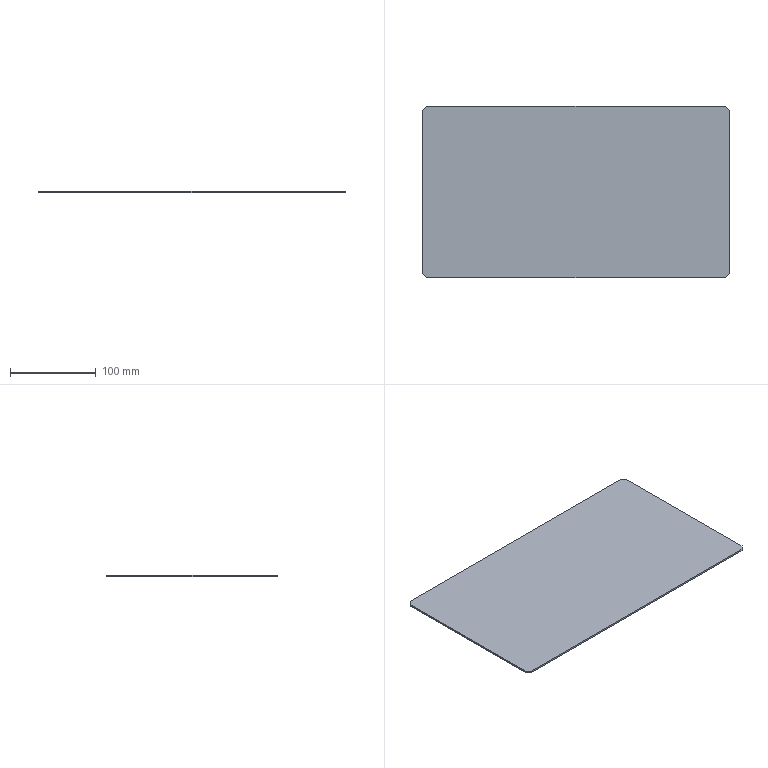Part | STEP file | PN_0042 | 1 solid | 10 faces | box 358 x 200 x 2 mm | volume 143100 mm3 | plane 10
STEP:
#1=CARTESIAN_POINT('',(0.,0.,0.));
#2=DIRECTION('',(0.,0.,1.));
#3=DIRECTION('',(1.,0.,0.));
#4=AXIS2_PLACEMENT_3D('',#1,#2,#3);
#5=CARTESIAN_POINT('',(179.,-95.,2.));
#6=VERTEX_POINT('',#5);
#7=CARTESIAN_POINT('',(179.,95.,2.));
#8=VERTEX_POINT('',#7);
#9=CARTESIAN_POINT('',(179.,100.,2.));
#10=DIRECTION('',(0.,1.,0.));
#11=VECTOR('',#10,1.);
#12=LINE('',#9,#11);
#13=CARTESIAN_POINT('',(179.,100.,2.));
#14=DIRECTION('',(-1.,0.,0.));
#15=DIRECTION('',(0.,-1.,0.));
#16=AXIS2_PLACEMENT_3D('',#13,#14,#15);
#17=PLANE('',#16);
#18=CARTESIAN_POINT('',(0.,0.));
#19=DIRECTION('',(-1.,0.));
#20=VECTOR('',#19,1.);
#21=LINE('',#18,#20);
#22=(GEOMETRIC_REPRESENTATION_CONTEXT(2)PARAMETRIC_REPRESENTATION_CONTEXT()REPRESENTATION_CONTEXT('',''));
#23=DEFINITIONAL_REPRESENTATION('',(#21),#22);
#24=PCURVE('',#17,#23);
#25=CARTESIAN_POINT('',(179.,-100.,2.));
#26=DIRECTION('',(0.,0.,1.));
#27=DIRECTION('',(1.,0.,0.));
#28=AXIS2_PLACEMENT_3D('',#25,#26,#27);
#29=PLANE('',#28);
#30=CARTESIAN_POINT('',(0.,200.));
#31=DIRECTION('',(0.,1.));
#32=VECTOR('',#31,1.);
#33=LINE('',#30,#32);
#34=(GEOMETRIC_REPRESENTATION_CONTEXT(2)PARAMETRIC_REPRESENTATION_CONTEXT()REPRESENTATION_CONTEXT('',''));
#35=DEFINITIONAL_REPRESENTATION('',(#33),#34);
#36=PCURVE('',#29,#35);
#37=SURFACE_CURVE('',#12,(#24,#36),.PCURVE_S1.);
#38=EDGE_CURVE('',#6,#8,#37,.T.);
#39=ORIENTED_EDGE('',*,*,#38,.F.);
#40=CARTESIAN_POINT('',(179.,-95.,0.));
#41=VERTEX_POINT('',#40);
#42=CARTESIAN_POINT('',(179.,-95.,2.));
#43=DIRECTION('',(0.,0.,-1.));
#44=VECTOR('',#43,1.);
#45=LINE('',#42,#44);
#46=CARTESIAN_POINT('',(195.,0.));
#47=DIRECTION('',(0.,-1.));
#48=VECTOR('',#47,1.);
#49=LINE('',#46,#48);
#50=(GEOMETRIC_REPRESENTATION_CONTEXT(2)PARAMETRIC_REPRESENTATION_CONTEXT()REPRESENTATION_CONTEXT('',''));
#51=DEFINITIONAL_REPRESENTATION('',(#49),#50);
#52=PCURVE('',#17,#51);
#53=CARTESIAN_POINT('',(179.,-95.,2.));
#54=DIRECTION('',(-0.7071,0.7071,0.));
#55=DIRECTION('',(-0.7071,-0.7071,0.));
#56=AXIS2_PLACEMENT_3D('',#53,#54,#55);
#57=PLANE('',#56);
#58=CARTESIAN_POINT('',(0.,0.));
#59=DIRECTION('',(0.,-1.));
#60=VECTOR('',#59,1.);
#61=LINE('',#58,#60);
#62=(GEOMETRIC_REPRESENTATION_CONTEXT(2)PARAMETRIC_REPRESENTATION_CONTEXT()REPRESENTATION_CONTEXT('',''));
#63=DEFINITIONAL_REPRESENTATION('',(#61),#62);
#64=PCURVE('',#57,#63);
#65=SURFACE_CURVE('',#45,(#52,#64),.PCURVE_S1.);
#66=EDGE_CURVE('',#6,#41,#65,.T.);
#67=ORIENTED_EDGE('',*,*,#66,.T.);
#68=CARTESIAN_POINT('',(179.,95.,0.));
#69=VERTEX_POINT('',#68);
#70=CARTESIAN_POINT('',(179.,100.,0.));
#71=DIRECTION('',(0.,1.,0.));
#72=VECTOR('',#71,1.);
#73=LINE('',#70,#72);
#74=CARTESIAN_POINT('',(0.,-2.));
#75=DIRECTION('',(-1.,0.));
#76=VECTOR('',#75,1.);
#77=LINE('',#74,#76);
#78=(GEOMETRIC_REPRESENTATION_CONTEXT(2)PARAMETRIC_REPRESENTATION_CONTEXT()REPRESENTATION_CONTEXT('',''));
#79=DEFINITIONAL_REPRESENTATION('',(#77),#78);
#80=PCURVE('',#17,#79);
#81=CARTESIAN_POINT('',(179.,-100.,0.));
#82=DIRECTION('',(0.,0.,1.));
#83=DIRECTION('',(1.,0.,0.));
#84=AXIS2_PLACEMENT_3D('',#81,#82,#83);
#85=PLANE('',#84);
#86=CARTESIAN_POINT('',(0.,200.));
#87=DIRECTION('',(0.,1.));
#88=VECTOR('',#87,1.);
#89=LINE('',#86,#88);
#90=(GEOMETRIC_REPRESENTATION_CONTEXT(2)PARAMETRIC_REPRESENTATION_CONTEXT()REPRESENTATION_CONTEXT('',''));
#91=DEFINITIONAL_REPRESENTATION('',(#89),#90);
#92=PCURVE('',#85,#91);
#93=SURFACE_CURVE('',#73,(#80,#92),.PCURVE_S1.);
#94=EDGE_CURVE('',#41,#69,#93,.T.);
#95=ORIENTED_EDGE('',*,*,#94,.T.);
#96=CARTESIAN_POINT('',(179.,95.,2.));
#97=DIRECTION('',(0.,0.,1.));
#98=VECTOR('',#97,1.);
#99=LINE('',#96,#98);
#100=CARTESIAN_POINT('',(5.,0.));
#101=DIRECTION('',(0.,1.));
#102=VECTOR('',#101,1.);
#103=LINE('',#100,#102);
#104=(GEOMETRIC_REPRESENTATION_CONTEXT(2)PARAMETRIC_REPRESENTATION_CONTEXT()REPRESENTATION_CONTEXT('',''));
#105=DEFINITIONAL_REPRESENTATION('',(#103),#104);
#106=PCURVE('',#17,#105);
#107=CARTESIAN_POINT('',(174.,100.,2.));
#108=DIRECTION('',(-0.7071,-0.7071,0.));
#109=DIRECTION('',(0.7071,-0.7071,0.));
#110=AXIS2_PLACEMENT_3D('',#107,#108,#109);
#111=PLANE('',#110);
#112=CARTESIAN_POINT('',(7.071,0.));
#113=DIRECTION('',(0.,1.));
#114=VECTOR('',#113,1.);
#115=LINE('',#112,#114);
#116=(GEOMETRIC_REPRESENTATION_CONTEXT(2)PARAMETRIC_REPRESENTATION_CONTEXT()REPRESENTATION_CONTEXT('',''));
#117=DEFINITIONAL_REPRESENTATION('',(#115),#116);
#118=PCURVE('',#111,#117);
#119=SURFACE_CURVE('',#99,(#106,#118),.PCURVE_S1.);
#120=EDGE_CURVE('',#69,#8,#119,.T.);
#121=ORIENTED_EDGE('',*,*,#120,.T.);
#122=EDGE_LOOP('',(#39,#67,#95,#121));
#123=FACE_BOUND('',#122,.T.);
#124=ADVANCED_FACE('',(#123),#17,.F.);
#125=CARTESIAN_POINT('',(174.,100.,0.));
#126=VERTEX_POINT('',#125);
#127=CARTESIAN_POINT('',(-174.,100.,0.));
#128=VERTEX_POINT('',#127);
#129=CARTESIAN_POINT('',(-179.,100.,0.));
#130=DIRECTION('',(-1.,0.,0.));
#131=VECTOR('',#130,1.);
#132=LINE('',#129,#131);
#133=CARTESIAN_POINT('',(-179.,100.,2.));
#134=DIRECTION('',(0.,-1.,0.));
#135=DIRECTION('',(0.,0.,-1.));
#136=AXIS2_PLACEMENT_3D('',#133,#134,#135);
#137=PLANE('',#136);
#138=CARTESIAN_POINT('',(2.,0.));
#139=DIRECTION('',(0.,-1.));
#140=VECTOR('',#139,1.);
#141=LINE('',#138,#140);
#142=(GEOMETRIC_REPRESENTATION_CONTEXT(2)PARAMETRIC_REPRESENTATION_CONTEXT()REPRESENTATION_CONTEXT('',''));
#143=DEFINITIONAL_REPRESENTATION('',(#141),#142);
#144=PCURVE('',#137,#143);
#145=CARTESIAN_POINT('',(-358.,200.));
#146=DIRECTION('',(-1.,0.));
#147=VECTOR('',#146,1.);
#148=LINE('',#145,#147);
#149=(GEOMETRIC_REPRESENTATION_CONTEXT(2)PARAMETRIC_REPRESENTATION_CONTEXT()REPRESENTATION_CONTEXT('',''));
#150=DEFINITIONAL_REPRESENTATION('',(#148),#149);
#151=PCURVE('',#85,#150);
#152=SURFACE_CURVE('',#132,(#144,#151),.PCURVE_S1.);
#153=EDGE_CURVE('',#126,#128,#152,.T.);
#154=ORIENTED_EDGE('',*,*,#153,.T.);
#155=CARTESIAN_POINT('',(-174.,100.,2.));
#156=VERTEX_POINT('',#155);
#157=CARTESIAN_POINT('',(-174.,100.,2.));
#158=DIRECTION('',(0.,0.,1.));
#159=VECTOR('',#158,1.);
#160=LINE('',#157,#159);
#161=CARTESIAN_POINT('',(0.,5.));
#162=DIRECTION('',(-1.,0.));
#163=VECTOR('',#162,1.);
#164=LINE('',#161,#163);
#165=(GEOMETRIC_REPRESENTATION_CONTEXT(2)PARAMETRIC_REPRESENTATION_CONTEXT()REPRESENTATION_CONTEXT('',''));
#166=DEFINITIONAL_REPRESENTATION('',(#164),#165);
#167=PCURVE('',#137,#166);
#168=CARTESIAN_POINT('',(-179.,95.,2.));
#169=DIRECTION('',(0.7071,-0.7071,0.));
#170=DIRECTION('',(0.7071,0.7071,0.));
#171=AXIS2_PLACEMENT_3D('',#168,#169,#170);
#172=PLANE('',#171);
#173=CARTESIAN_POINT('',(7.071,0.));
#174=DIRECTION('',(0.,1.));
#175=VECTOR('',#174,1.);
#176=LINE('',#173,#175);
#177=(GEOMETRIC_REPRESENTATION_CONTEXT(2)PARAMETRIC_REPRESENTATION_CONTEXT()REPRESENTATION_CONTEXT('',''));
#178=DEFINITIONAL_REPRESENTATION('',(#176),#177);
#179=PCURVE('',#172,#178);
#180=SURFACE_CURVE('',#160,(#167,#179),.PCURVE_S1.);
#181=EDGE_CURVE('',#128,#156,#180,.T.);
#182=ORIENTED_EDGE('',*,*,#181,.T.);
#183=CARTESIAN_POINT('',(174.,100.,2.));
#184=VERTEX_POINT('',#183);
#185=CARTESIAN_POINT('',(-179.,100.,2.));
#186=DIRECTION('',(-1.,0.,0.));
#187=VECTOR('',#186,1.);
#188=LINE('',#185,#187);
#189=CARTESIAN_POINT('',(0.,0.));
#190=DIRECTION('',(0.,-1.));
#191=VECTOR('',#190,1.);
#192=LINE('',#189,#191);
#193=(GEOMETRIC_REPRESENTATION_CONTEXT(2)PARAMETRIC_REPRESENTATION_CONTEXT()REPRESENTATION_CONTEXT('',''));
#194=DEFINITIONAL_REPRESENTATION('',(#192),#193);
#195=PCURVE('',#137,#194);
#196=CARTESIAN_POINT('',(-358.,200.));
#197=DIRECTION('',(-1.,0.));
#198=VECTOR('',#197,1.);
#199=LINE('',#196,#198);
#200=(GEOMETRIC_REPRESENTATION_CONTEXT(2)PARAMETRIC_REPRESENTATION_CONTEXT()REPRESENTATION_CONTEXT('',''));
#201=DEFINITIONAL_REPRESENTATION('',(#199),#200);
#202=PCURVE('',#29,#201);
#203=SURFACE_CURVE('',#188,(#195,#202),.PCURVE_S1.);
#204=EDGE_CURVE('',#184,#156,#203,.T.);
#205=ORIENTED_EDGE('',*,*,#204,.F.);
#206=CARTESIAN_POINT('',(174.,100.,2.));
#207=DIRECTION('',(0.,0.,-1.));
#208=VECTOR('',#207,1.);
#209=LINE('',#206,#208);
#210=CARTESIAN_POINT('',(0.,353.));
#211=DIRECTION('',(1.,0.));
#212=VECTOR('',#211,1.);
#213=LINE('',#210,#212);
#214=(GEOMETRIC_REPRESENTATION_CONTEXT(2)PARAMETRIC_REPRESENTATION_CONTEXT()REPRESENTATION_CONTEXT('',''));
#215=DEFINITIONAL_REPRESENTATION('',(#213),#214);
#216=PCURVE('',#137,#215);
#217=CARTESIAN_POINT('',(0.,0.));
#218=DIRECTION('',(0.,-1.));
#219=VECTOR('',#218,1.);
#220=LINE('',#217,#219);
#221=(GEOMETRIC_REPRESENTATION_CONTEXT(2)PARAMETRIC_REPRESENTATION_CONTEXT()REPRESENTATION_CONTEXT('',''));
#222=DEFINITIONAL_REPRESENTATION('',(#220),#221);
#223=PCURVE('',#111,#222);
#224=SURFACE_CURVE('',#209,(#216,#223),.PCURVE_S1.);
#225=EDGE_CURVE('',#184,#126,#224,.T.);
#226=ORIENTED_EDGE('',*,*,#225,.T.);
#227=EDGE_LOOP('',(#154,#182,#205,#226));
#228=FACE_BOUND('',#227,.T.);
#229=ADVANCED_FACE('',(#228),#137,.F.);
#230=CARTESIAN_POINT('',(-179.,95.,0.));
#231=VERTEX_POINT('',#230);
#232=CARTESIAN_POINT('',(-179.,-95.,0.));
#233=VERTEX_POINT('',#232);
#234=CARTESIAN_POINT('',(-179.,100.,0.));
#235=DIRECTION('',(0.,-1.,0.));
#236=VECTOR('',#235,1.);
#237=LINE('',#234,#236);
#238=CARTESIAN_POINT('',(-179.,100.,2.));
#239=DIRECTION('',(1.,0.,0.));
#240=DIRECTION('',(0.,1.,0.));
#241=AXIS2_PLACEMENT_3D('',#238,#239,#240);
#242=PLANE('',#241);
#243=CARTESIAN_POINT('',(0.,-2.));
#244=DIRECTION('',(-1.,0.));
#245=VECTOR('',#244,1.);
#246=LINE('',#243,#245);
#247=(GEOMETRIC_REPRESENTATION_CONTEXT(2)PARAMETRIC_REPRESENTATION_CONTEXT()REPRESENTATION_CONTEXT('',''));
#248=DEFINITIONAL_REPRESENTATION('',(#246),#247);
#249=PCURVE('',#242,#248);
#250=CARTESIAN_POINT('',(-358.,200.));
#251=DIRECTION('',(0.,-1.));
#252=VECTOR('',#251,1.);
#253=LINE('',#250,#252);
#254=(GEOMETRIC_REPRESENTATION_CONTEXT(2)PARAMETRIC_REPRESENTATION_CONTEXT()REPRESENTATION_CONTEXT('',''));
#255=DEFINITIONAL_REPRESENTATION('',(#253),#254);
#256=PCURVE('',#85,#255);
#257=SURFACE_CURVE('',#237,(#249,#256),.PCURVE_S1.);
#258=EDGE_CURVE('',#231,#233,#257,.T.);
#259=ORIENTED_EDGE('',*,*,#258,.T.);
#260=CARTESIAN_POINT('',(-179.,-95.,2.));
#261=VERTEX_POINT('',#260);
#262=CARTESIAN_POINT('',(-179.,-95.,2.));
#263=DIRECTION('',(0.,0.,1.));
#264=VECTOR('',#263,1.);
#265=LINE('',#262,#264);
#266=CARTESIAN_POINT('',(-195.,0.));
#267=DIRECTION('',(0.,1.));
#268=VECTOR('',#267,1.);
#269=LINE('',#266,#268);
#270=(GEOMETRIC_REPRESENTATION_CONTEXT(2)PARAMETRIC_REPRESENTATION_CONTEXT()REPRESENTATION_CONTEXT('',''));
#271=DEFINITIONAL_REPRESENTATION('',(#269),#270);
#272=PCURVE('',#242,#271);
#273=CARTESIAN_POINT('',(-174.,-100.,2.));
#274=DIRECTION('',(0.7071,0.7071,0.));
#275=DIRECTION('',(-0.7071,0.7071,0.));
#276=AXIS2_PLACEMENT_3D('',#273,#274,#275);
#277=PLANE('',#276);
#278=CARTESIAN_POINT('',(7.071,0.));
#279=DIRECTION('',(0.,1.));
#280=VECTOR('',#279,1.);
#281=LINE('',#278,#280);
#282=(GEOMETRIC_REPRESENTATION_CONTEXT(2)PARAMETRIC_REPRESENTATION_CONTEXT()REPRESENTATION_CONTEXT('',''));
#283=DEFINITIONAL_REPRESENTATION('',(#281),#282);
#284=PCURVE('',#277,#283);
#285=SURFACE_CURVE('',#265,(#272,#284),.PCURVE_S1.);
#286=EDGE_CURVE('',#233,#261,#285,.T.);
#287=ORIENTED_EDGE('',*,*,#286,.T.);
#288=CARTESIAN_POINT('',(-179.,95.,2.));
#289=VERTEX_POINT('',#288);
#290=CARTESIAN_POINT('',(-179.,100.,2.));
#291=DIRECTION('',(0.,-1.,0.));
#292=VECTOR('',#291,1.);
#293=LINE('',#290,#292);
#294=CARTESIAN_POINT('',(0.,0.));
#295=DIRECTION('',(-1.,0.));
#296=VECTOR('',#295,1.);
#297=LINE('',#294,#296);
#298=(GEOMETRIC_REPRESENTATION_CONTEXT(2)PARAMETRIC_REPRESENTATION_CONTEXT()REPRESENTATION_CONTEXT('',''));
#299=DEFINITIONAL_REPRESENTATION('',(#297),#298);
#300=PCURVE('',#242,#299);
#301=CARTESIAN_POINT('',(-358.,200.));
#302=DIRECTION('',(0.,-1.));
#303=VECTOR('',#302,1.);
#304=LINE('',#301,#303);
#305=(GEOMETRIC_REPRESENTATION_CONTEXT(2)PARAMETRIC_REPRESENTATION_CONTEXT()REPRESENTATION_CONTEXT('',''));
#306=DEFINITIONAL_REPRESENTATION('',(#304),#305);
#307=PCURVE('',#29,#306);
#308=SURFACE_CURVE('',#293,(#300,#307),.PCURVE_S1.);
#309=EDGE_CURVE('',#289,#261,#308,.T.);
#310=ORIENTED_EDGE('',*,*,#309,.F.);
#311=CARTESIAN_POINT('',(-179.,95.,2.));
#312=DIRECTION('',(0.,0.,-1.));
#313=VECTOR('',#312,1.);
#314=LINE('',#311,#313);
#315=CARTESIAN_POINT('',(-5.,0.));
#316=DIRECTION('',(0.,-1.));
#317=VECTOR('',#316,1.);
#318=LINE('',#315,#317);
#319=(GEOMETRIC_REPRESENTATION_CONTEXT(2)PARAMETRIC_REPRESENTATION_CONTEXT()REPRESENTATION_CONTEXT('',''));
#320=DEFINITIONAL_REPRESENTATION('',(#318),#319);
#321=PCURVE('',#242,#320);
#322=CARTESIAN_POINT('',(0.,0.));
#323=DIRECTION('',(0.,-1.));
#324=VECTOR('',#323,1.);
#325=LINE('',#322,#324);
#326=(GEOMETRIC_REPRESENTATION_CONTEXT(2)PARAMETRIC_REPRESENTATION_CONTEXT()REPRESENTATION_CONTEXT('',''));
#327=DEFINITIONAL_REPRESENTATION('',(#325),#326);
#328=PCURVE('',#172,#327);
#329=SURFACE_CURVE('',#314,(#321,#328),.PCURVE_S1.);
#330=EDGE_CURVE('',#289,#231,#329,.T.);
#331=ORIENTED_EDGE('',*,*,#330,.T.);
#332=EDGE_LOOP('',(#259,#287,#310,#331));
#333=FACE_BOUND('',#332,.T.);
#334=ADVANCED_FACE('',(#333),#242,.F.);
#335=CARTESIAN_POINT('',(-174.,-100.,2.));
#336=VERTEX_POINT('',#335);
#337=CARTESIAN_POINT('',(174.,-100.,2.));
#338=VERTEX_POINT('',#337);
#339=CARTESIAN_POINT('',(-179.,-100.,2.));
#340=DIRECTION('',(1.,0.,0.));
#341=VECTOR('',#340,1.);
#342=LINE('',#339,#341);
#343=CARTESIAN_POINT('',(-179.,-100.,2.));
#344=DIRECTION('',(0.,1.,0.));
#345=DIRECTION('',(0.,0.,1.));
#346=AXIS2_PLACEMENT_3D('',#343,#344,#345);
#347=PLANE('',#346);
#348=CARTESIAN_POINT('',(0.,0.));
#349=DIRECTION('',(0.,1.));
#350=VECTOR('',#349,1.);
#351=LINE('',#348,#350);
#352=(GEOMETRIC_REPRESENTATION_CONTEXT(2)PARAMETRIC_REPRESENTATION_CONTEXT()REPRESENTATION_CONTEXT('',''));
#353=DEFINITIONAL_REPRESENTATION('',(#351),#352);
#354=PCURVE('',#347,#353);
#355=CARTESIAN_POINT('',(-358.,0.));
#356=DIRECTION('',(1.,0.));
#357=VECTOR('',#356,1.);
#358=LINE('',#355,#357);
#359=(GEOMETRIC_REPRESENTATION_CONTEXT(2)PARAMETRIC_REPRESENTATION_CONTEXT()REPRESENTATION_CONTEXT('',''));
#360=DEFINITIONAL_REPRESENTATION('',(#358),#359);
#361=PCURVE('',#29,#360);
#362=SURFACE_CURVE('',#342,(#354,#361),.PCURVE_S1.);
#363=EDGE_CURVE('',#336,#338,#362,.T.);
#364=ORIENTED_EDGE('',*,*,#363,.F.);
#365=CARTESIAN_POINT('',(-174.,-100.,0.));
#366=VERTEX_POINT('',#365);
#367=CARTESIAN_POINT('',(-174.,-100.,2.));
#368=DIRECTION('',(0.,0.,-1.));
#369=VECTOR('',#368,1.);
#370=LINE('',#367,#369);
#371=CARTESIAN_POINT('',(0.,5.));
#372=DIRECTION('',(-1.,0.));
#373=VECTOR('',#372,1.);
#374=LINE('',#371,#373);
#375=(GEOMETRIC_REPRESENTATION_CONTEXT(2)PARAMETRIC_REPRESENTATION_CONTEXT()REPRESENTATION_CONTEXT('',''));
#376=DEFINITIONAL_REPRESENTATION('',(#374),#375);
#377=PCURVE('',#347,#376);
#378=CARTESIAN_POINT('',(0.,0.));
#379=DIRECTION('',(0.,-1.));
#380=VECTOR('',#379,1.);
#381=LINE('',#378,#380);
#382=(GEOMETRIC_REPRESENTATION_CONTEXT(2)PARAMETRIC_REPRESENTATION_CONTEXT()REPRESENTATION_CONTEXT('',''));
#383=DEFINITIONAL_REPRESENTATION('',(#381),#382);
#384=PCURVE('',#277,#383);
#385=SURFACE_CURVE('',#370,(#377,#384),.PCURVE_S1.);
#386=EDGE_CURVE('',#336,#366,#385,.T.);
#387=ORIENTED_EDGE('',*,*,#386,.T.);
#388=CARTESIAN_POINT('',(174.,-100.,0.));
#389=VERTEX_POINT('',#388);
#390=CARTESIAN_POINT('',(-179.,-100.,0.));
#391=DIRECTION('',(1.,0.,0.));
#392=VECTOR('',#391,1.);
#393=LINE('',#390,#392);
#394=CARTESIAN_POINT('',(-2.,0.));
#395=DIRECTION('',(0.,1.));
#396=VECTOR('',#395,1.);
#397=LINE('',#394,#396);
#398=(GEOMETRIC_REPRESENTATION_CONTEXT(2)PARAMETRIC_REPRESENTATION_CONTEXT()REPRESENTATION_CONTEXT('',''));
#399=DEFINITIONAL_REPRESENTATION('',(#397),#398);
#400=PCURVE('',#347,#399);
#401=CARTESIAN_POINT('',(-358.,0.));
#402=DIRECTION('',(1.,0.));
#403=VECTOR('',#402,1.);
#404=LINE('',#401,#403);
#405=(GEOMETRIC_REPRESENTATION_CONTEXT(2)PARAMETRIC_REPRESENTATION_CONTEXT()REPRESENTATION_CONTEXT('',''));
#406=DEFINITIONAL_REPRESENTATION('',(#404),#405);
#407=PCURVE('',#85,#406);
#408=SURFACE_CURVE('',#393,(#400,#407),.PCURVE_S1.);
#409=EDGE_CURVE('',#366,#389,#408,.T.);
#410=ORIENTED_EDGE('',*,*,#409,.T.);
#411=CARTESIAN_POINT('',(174.,-100.,2.));
#412=DIRECTION('',(0.,0.,1.));
#413=VECTOR('',#412,1.);
#414=LINE('',#411,#413);
#415=CARTESIAN_POINT('',(0.,353.));
#416=DIRECTION('',(1.,0.));
#417=VECTOR('',#416,1.);
#418=LINE('',#415,#417);
#419=(GEOMETRIC_REPRESENTATION_CONTEXT(2)PARAMETRIC_REPRESENTATION_CONTEXT()REPRESENTATION_CONTEXT('',''));
#420=DEFINITIONAL_REPRESENTATION('',(#418),#419);
#421=PCURVE('',#347,#420);
#422=CARTESIAN_POINT('',(7.071,0.));
#423=DIRECTION('',(0.,1.));
#424=VECTOR('',#423,1.);
#425=LINE('',#422,#424);
#426=(GEOMETRIC_REPRESENTATION_CONTEXT(2)PARAMETRIC_REPRESENTATION_CONTEXT()REPRESENTATION_CONTEXT('',''));
#427=DEFINITIONAL_REPRESENTATION('',(#425),#426);
#428=PCURVE('',#57,#427);
#429=SURFACE_CURVE('',#414,(#421,#428),.PCURVE_S1.);
#430=EDGE_CURVE('',#389,#338,#429,.T.);
#431=ORIENTED_EDGE('',*,*,#430,.T.);
#432=EDGE_LOOP('',(#364,#387,#410,#431));
#433=FACE_BOUND('',#432,.T.);
#434=ADVANCED_FACE('',(#433),#347,.F.);
#435=ORIENTED_EDGE('',*,*,#309,.T.);
#436=CARTESIAN_POINT('',(2.5,-276.5,2.));
#437=DIRECTION('',(0.7071,-0.7071,0.));
#438=VECTOR('',#437,1.);
#439=LINE('',#436,#438);
#440=CARTESIAN_POINT('',(-176.5,-176.5));
#441=DIRECTION('',(0.7071,-0.7071));
#442=VECTOR('',#441,1.);
#443=LINE('',#440,#442);
#444=(GEOMETRIC_REPRESENTATION_CONTEXT(2)PARAMETRIC_REPRESENTATION_CONTEXT()REPRESENTATION_CONTEXT('',''));
#445=DEFINITIONAL_REPRESENTATION('',(#443),#444);
#446=PCURVE('',#29,#445);
#447=CARTESIAN_POINT('',(-249.609,0.));
#448=DIRECTION('',(-1.,0.));
#449=VECTOR('',#448,1.);
#450=LINE('',#447,#449);
#451=(GEOMETRIC_REPRESENTATION_CONTEXT(2)PARAMETRIC_REPRESENTATION_CONTEXT()REPRESENTATION_CONTEXT('',''));
#452=DEFINITIONAL_REPRESENTATION('',(#450),#451);
#453=PCURVE('',#277,#452);
#454=SURFACE_CURVE('',#439,(#446,#453),.PCURVE_S1.);
#455=EDGE_CURVE('',#261,#336,#454,.T.);
#456=ORIENTED_EDGE('',*,*,#455,.T.);
#457=ORIENTED_EDGE('',*,*,#363,.T.);
#458=CARTESIAN_POINT('',(176.5,-97.5,2.));
#459=DIRECTION('',(0.7071,0.7071,0.));
#460=VECTOR('',#459,1.);
#461=LINE('',#458,#460);
#462=CARTESIAN_POINT('',(-2.5,2.5));
#463=DIRECTION('',(0.7071,0.7071));
#464=VECTOR('',#463,1.);
#465=LINE('',#462,#464);
#466=(GEOMETRIC_REPRESENTATION_CONTEXT(2)PARAMETRIC_REPRESENTATION_CONTEXT()REPRESENTATION_CONTEXT('',''));
#467=DEFINITIONAL_REPRESENTATION('',(#465),#466);
#468=PCURVE('',#29,#467);
#469=CARTESIAN_POINT('',(3.536,0.));
#470=DIRECTION('',(-1.,0.));
#471=VECTOR('',#470,1.);
#472=LINE('',#469,#471);
#473=(GEOMETRIC_REPRESENTATION_CONTEXT(2)PARAMETRIC_REPRESENTATION_CONTEXT()REPRESENTATION_CONTEXT('',''));
#474=DEFINITIONAL_REPRESENTATION('',(#472),#473);
#475=PCURVE('',#57,#474);
#476=SURFACE_CURVE('',#461,(#468,#475),.PCURVE_S1.);
#477=EDGE_CURVE('',#338,#6,#476,.T.);
#478=ORIENTED_EDGE('',*,*,#477,.T.);
#479=ORIENTED_EDGE('',*,*,#38,.T.);
#480=CARTESIAN_POINT('',(276.5,-2.5,2.));
#481=DIRECTION('',(-0.7071,0.7071,0.));
#482=VECTOR('',#481,1.);
#483=LINE('',#480,#482);
#484=CARTESIAN_POINT('',(97.5,97.5));
#485=DIRECTION('',(-0.7071,0.7071));
#486=VECTOR('',#485,1.);
#487=LINE('',#484,#486);
#488=(GEOMETRIC_REPRESENTATION_CONTEXT(2)PARAMETRIC_REPRESENTATION_CONTEXT()REPRESENTATION_CONTEXT('',''));
#489=DEFINITIONAL_REPRESENTATION('',(#487),#488);
#490=PCURVE('',#29,#489);
#491=CARTESIAN_POINT('',(144.957,0.));
#492=DIRECTION('',(-1.,0.));
#493=VECTOR('',#492,1.);
#494=LINE('',#491,#493);
#495=(GEOMETRIC_REPRESENTATION_CONTEXT(2)PARAMETRIC_REPRESENTATION_CONTEXT()REPRESENTATION_CONTEXT('',''));
#496=DEFINITIONAL_REPRESENTATION('',(#494),#495);
#497=PCURVE('',#111,#496);
#498=SURFACE_CURVE('',#483,(#490,#497),.PCURVE_S1.);
#499=EDGE_CURVE('',#8,#184,#498,.T.);
#500=ORIENTED_EDGE('',*,*,#499,.T.);
#501=ORIENTED_EDGE('',*,*,#204,.T.);
#502=CARTESIAN_POINT('',(-97.5,176.5,2.));
#503=DIRECTION('',(-0.7071,-0.7071,0.));
#504=VECTOR('',#503,1.);
#505=LINE('',#502,#504);
#506=CARTESIAN_POINT('',(-276.5,276.5));
#507=DIRECTION('',(-0.7071,-0.7071));
#508=VECTOR('',#507,1.);
#509=LINE('',#506,#508);
#510=(GEOMETRIC_REPRESENTATION_CONTEXT(2)PARAMETRIC_REPRESENTATION_CONTEXT()REPRESENTATION_CONTEXT('',''));
#511=DEFINITIONAL_REPRESENTATION('',(#509),#510);
#512=PCURVE('',#29,#511);
#513=CARTESIAN_POINT('',(115.258,0.));
#514=DIRECTION('',(-1.,0.));
#515=VECTOR('',#514,1.);
#516=LINE('',#513,#515);
#517=(GEOMETRIC_REPRESENTATION_CONTEXT(2)PARAMETRIC_REPRESENTATION_CONTEXT()REPRESENTATION_CONTEXT('',''));
#518=DEFINITIONAL_REPRESENTATION('',(#516),#517);
#519=PCURVE('',#172,#518);
#520=SURFACE_CURVE('',#505,(#512,#519),.PCURVE_S1.);
#521=EDGE_CURVE('',#156,#289,#520,.T.);
#522=ORIENTED_EDGE('',*,*,#521,.T.);
#523=EDGE_LOOP('',(#435,#456,#457,#478,#479,#500,#501,#522));
#524=FACE_BOUND('',#523,.T.);
#525=ADVANCED_FACE('',(#524),#29,.T.);
#526=ORIENTED_EDGE('',*,*,#409,.F.);
#527=CARTESIAN_POINT('',(-174.,-100.,0.));
#528=DIRECTION('',(-0.7071,0.7071,0.));
#529=VECTOR('',#528,1.);
#530=LINE('',#527,#529);
#531=CARTESIAN_POINT('',(-353.,0.));
#532=DIRECTION('',(-0.7071,0.7071));
#533=VECTOR('',#532,1.);
#534=LINE('',#531,#533);
#535=(GEOMETRIC_REPRESENTATION_CONTEXT(2)PARAMETRIC_REPRESENTATION_CONTEXT()REPRESENTATION_CONTEXT('',''));
#536=DEFINITIONAL_REPRESENTATION('',(#534),#535);
#537=PCURVE('',#85,#536);
#538=CARTESIAN_POINT('',(0.,-2.));
#539=DIRECTION('',(1.,0.));
#540=VECTOR('',#539,1.);
#541=LINE('',#538,#540);
#542=(GEOMETRIC_REPRESENTATION_CONTEXT(2)PARAMETRIC_REPRESENTATION_CONTEXT()REPRESENTATION_CONTEXT('',''));
#543=DEFINITIONAL_REPRESENTATION('',(#541),#542);
#544=PCURVE('',#277,#543);
#545=SURFACE_CURVE('',#530,(#537,#544),.PCURVE_S1.);
#546=EDGE_CURVE('',#366,#233,#545,.T.);
#547=ORIENTED_EDGE('',*,*,#546,.T.);
#548=ORIENTED_EDGE('',*,*,#258,.F.);
#549=CARTESIAN_POINT('',(-179.,95.,0.));
#550=DIRECTION('',(0.7071,0.7071,0.));
#551=VECTOR('',#550,1.);
#552=LINE('',#549,#551);
#553=CARTESIAN_POINT('',(-358.,195.));
#554=DIRECTION('',(0.7071,0.7071));
#555=VECTOR('',#554,1.);
#556=LINE('',#553,#555);
#557=(GEOMETRIC_REPRESENTATION_CONTEXT(2)PARAMETRIC_REPRESENTATION_CONTEXT()REPRESENTATION_CONTEXT('',''));
#558=DEFINITIONAL_REPRESENTATION('',(#556),#557);
#559=PCURVE('',#85,#558);
#560=CARTESIAN_POINT('',(0.,-2.));
#561=DIRECTION('',(1.,0.));
#562=VECTOR('',#561,1.);
#563=LINE('',#560,#562);
#564=(GEOMETRIC_REPRESENTATION_CONTEXT(2)PARAMETRIC_REPRESENTATION_CONTEXT()REPRESENTATION_CONTEXT('',''));
#565=DEFINITIONAL_REPRESENTATION('',(#563),#564);
#566=PCURVE('',#172,#565);
#567=SURFACE_CURVE('',#552,(#559,#566),.PCURVE_S1.);
#568=EDGE_CURVE('',#231,#128,#567,.T.);
#569=ORIENTED_EDGE('',*,*,#568,.T.);
#570=ORIENTED_EDGE('',*,*,#153,.F.);
#571=CARTESIAN_POINT('',(174.,100.,0.));
#572=DIRECTION('',(0.7071,-0.7071,0.));
#573=VECTOR('',#572,1.);
#574=LINE('',#571,#573);
#575=CARTESIAN_POINT('',(-5.,200.));
#576=DIRECTION('',(0.7071,-0.7071));
#577=VECTOR('',#576,1.);
#578=LINE('',#575,#577);
#579=(GEOMETRIC_REPRESENTATION_CONTEXT(2)PARAMETRIC_REPRESENTATION_CONTEXT()REPRESENTATION_CONTEXT('',''));
#580=DEFINITIONAL_REPRESENTATION('',(#578),#579);
#581=PCURVE('',#85,#580);
#582=CARTESIAN_POINT('',(0.,-2.));
#583=DIRECTION('',(1.,0.));
#584=VECTOR('',#583,1.);
#585=LINE('',#582,#584);
#586=(GEOMETRIC_REPRESENTATION_CONTEXT(2)PARAMETRIC_REPRESENTATION_CONTEXT()REPRESENTATION_CONTEXT('',''));
#587=DEFINITIONAL_REPRESENTATION('',(#585),#586);
#588=PCURVE('',#111,#587);
#589=SURFACE_CURVE('',#574,(#581,#588),.PCURVE_S1.);
#590=EDGE_CURVE('',#126,#69,#589,.T.);
#591=ORIENTED_EDGE('',*,*,#590,.T.);
#592=ORIENTED_EDGE('',*,*,#94,.F.);
#593=CARTESIAN_POINT('',(179.,-95.,0.));
#594=DIRECTION('',(-0.7071,-0.7071,0.));
#595=VECTOR('',#594,1.);
#596=LINE('',#593,#595);
#597=CARTESIAN_POINT('',(0.,5.));
#598=DIRECTION('',(-0.7071,-0.7071));
#599=VECTOR('',#598,1.);
#600=LINE('',#597,#599);
#601=(GEOMETRIC_REPRESENTATION_CONTEXT(2)PARAMETRIC_REPRESENTATION_CONTEXT()REPRESENTATION_CONTEXT('',''));
#602=DEFINITIONAL_REPRESENTATION('',(#600),#601);
#603=PCURVE('',#85,#602);
#604=CARTESIAN_POINT('',(0.,-2.));
#605=DIRECTION('',(1.,0.));
#606=VECTOR('',#605,1.);
#607=LINE('',#604,#606);
#608=(GEOMETRIC_REPRESENTATION_CONTEXT(2)PARAMETRIC_REPRESENTATION_CONTEXT()REPRESENTATION_CONTEXT('',''));
#609=DEFINITIONAL_REPRESENTATION('',(#607),#608);
#610=PCURVE('',#57,#609);
#611=SURFACE_CURVE('',#596,(#603,#610),.PCURVE_S1.);
#612=EDGE_CURVE('',#41,#389,#611,.T.);
#613=ORIENTED_EDGE('',*,*,#612,.T.);
#614=EDGE_LOOP('',(#526,#547,#548,#569,#570,#591,#592,#613));
#615=FACE_BOUND('',#614,.T.);
#616=ADVANCED_FACE('',(#615),#85,.F.);
#617=ORIENTED_EDGE('',*,*,#455,.F.);
#618=ORIENTED_EDGE('',*,*,#286,.F.);
#619=ORIENTED_EDGE('',*,*,#546,.F.);
#620=ORIENTED_EDGE('',*,*,#386,.F.);
#621=EDGE_LOOP('',(#617,#618,#619,#620));
#622=FACE_BOUND('',#621,.T.);
#623=ADVANCED_FACE('',(#622),#277,.F.);
#624=ORIENTED_EDGE('',*,*,#521,.F.);
#625=ORIENTED_EDGE('',*,*,#181,.F.);
#626=ORIENTED_EDGE('',*,*,#568,.F.);
#627=ORIENTED_EDGE('',*,*,#330,.F.);
#628=EDGE_LOOP('',(#624,#625,#626,#627));
#629=FACE_BOUND('',#628,.T.);
#630=ADVANCED_FACE('',(#629),#172,.F.);
#631=ORIENTED_EDGE('',*,*,#477,.F.);
#632=ORIENTED_EDGE('',*,*,#430,.F.);
#633=ORIENTED_EDGE('',*,*,#612,.F.);
#634=ORIENTED_EDGE('',*,*,#66,.F.);
#635=EDGE_LOOP('',(#631,#632,#633,#634));
#636=FACE_BOUND('',#635,.T.);
#637=ADVANCED_FACE('',(#636),#57,.F.);
#638=ORIENTED_EDGE('',*,*,#499,.F.);
#639=ORIENTED_EDGE('',*,*,#120,.F.);
#640=ORIENTED_EDGE('',*,*,#590,.F.);
#641=ORIENTED_EDGE('',*,*,#225,.F.);
#642=EDGE_LOOP('',(#638,#639,#640,#641));
#643=FACE_BOUND('',#642,.T.);
#644=ADVANCED_FACE('',(#643),#111,.F.);
#645=CLOSED_SHELL('',(#124,#229,#334,#434,#525,#616,#623,#630,#637,#644));
#646=MANIFOLD_SOLID_BREP('',#645);
#647=(LENGTH_UNIT()NAMED_UNIT(*)SI_UNIT(.MILLI.,.METRE.));
#648=UNCERTAINTY_MEASURE_WITH_UNIT(LENGTH_MEASURE(0.0000001),#647,'','');
#649=(NAMED_UNIT(*)PLANE_ANGLE_UNIT()SI_UNIT($,.RADIAN.));
#650=(NAMED_UNIT(*)SI_UNIT($,.STERADIAN.)SOLID_ANGLE_UNIT());
#651=(GEOMETRIC_REPRESENTATION_CONTEXT(3)GLOBAL_UNCERTAINTY_ASSIGNED_CONTEXT((#648))GLOBAL_UNIT_ASSIGNED_CONTEXT((#647,#649,#650))REPRESENTATION_CONTEXT('',''));
#652=ADVANCED_BREP_SHAPE_REPRESENTATION('',(#4,#646),#651);